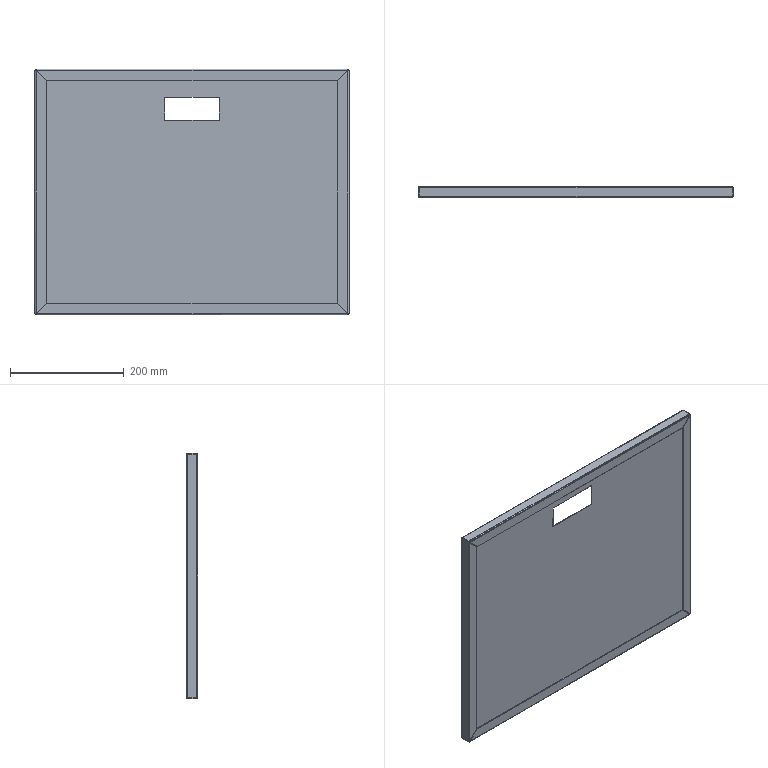Part | SolidWorks | features EdgeFlange 2, FlatPattern 1, ICE 1, SMBaseFlange 1, SheetMetal 1 | 1 solid | 74 faces | box 552 x 20 x 432 mm | volume 364714 mm3 | plane 42 | spline 16 | cylinder 16 | commonest cylinder face diameters 2 x8 4.4 x8